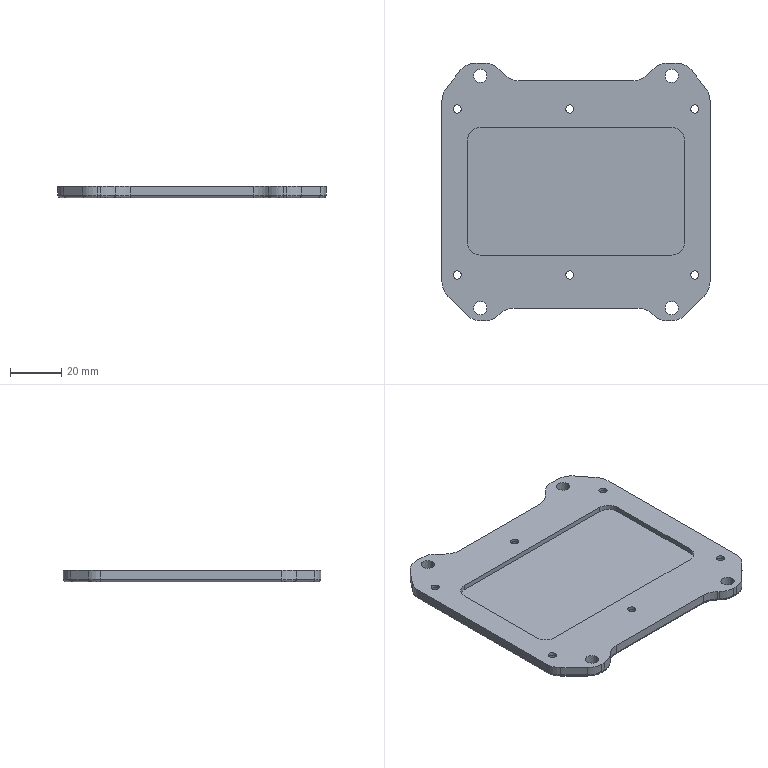NC program | NX | posted with a generic post | part box 105 x 101 x 4.5 mm
Whole program:
N10 G17 G21 G94 G90
(FLOOR_WALL_1 , TOOL : D80面刀)
N12 T01 M6
N14 G54
N16 G17 G0 G90 X-30.5 Y-95.5 S3500 M3
N18 G43 Z20. H1
N20 Z7.02
N22 G94 G1 Z4.02 F1000.
N24 Y-92.5
N26 Y92.5
N28 Y95.5
N30 Z7.02
N32 G0 Z20.
N34 X18.5 Y-95.5
N36 Z7.02
N38 G1 Z4.02
N40 Y-92.5
N42 Y92.5
N44 Y95.5
N46 Z7.02
N48 G0 Z20.
N50 X-30.5 Y-95.5
N52 Z6.04
N54 G1 Z3.04
N56 Y-92.5
N58 Y92.5
N60 Y95.5
N62 Z6.04
N64 G0 Z20.
N66 X18.5 Y-95.5
N68 Z6.04
N70 G1 Z3.04
N72 Y-92.5
N74 Y92.5
N76 Y95.5
N78 Z6.04
N80 G0 Z20.
N82 X-30.5 Y-95.5
N84 Z5.06
N86 G1 Z2.06
N88 Y-92.5
N90 Y92.5
N92 Y95.5
N94 Z5.06
N96 G0 Z20.
N98 X18.5 Y-95.5
N100 Z5.06
N102 G1 Z2.06
N104 Y-92.5
N106 Y92.5
N108 Y95.5
N110 Z5.06
N112 G0 Z20.
N114 X-30.5 Y-95.5
N116 Z4.08
N118 G1 Z1.08
N120 Y-92.5
N122 Y92.5
N124 Y95.5
N126 Z4.08
N128 G0 Z20.
N130 X18.5 Y-95.5
N132 Z4.08
N134 G1 Z1.08
N136 Y-92.5
N138 Y92.5
N140 Y95.5
N142 Z4.08
N144 G0 Z20.
N146 X-30.5 Y-95.5
N148 Z3.1
N150 G1 Z0.1
N152 Y-92.5
N154 Y92.5
N156 Y95.5
N158 Z3.1
N160 G0 Z20.
N162 X18.5 Y-95.5
N164 Z3.1
N166 G1 Z0.1
N168 Y-92.5
N170 Y92.5
N172 Y95.5
N174 Z3.1
N176 G0 Z20.
(FLOOR_WALL_1_COPY , TOOL : D80面刀)
N178 X-30.5 Y-95.5
N180 Z3.
N182 G1 Z0.
N184 Y-92.5
N186 Y92.5
N188 Y95.5
N190 Z3.
N192 G0 Z20.
N194 X18.5 Y-95.5
N196 Z3.
N198 G1 Z0.
N200 Y-92.5
N202 Y92.5
N204 Y95.5
N206 Z3.
N208 G0 Z20.
N210 M5
(PLANAR_MILL_2 , TOOL : D8-24-D8-60波刀)
N212 T02 M6
N214 G54
N216 G17 G0 G90 X2.576 Y17.778 S4500 M3
N218 G43 Z20. H2
N220 Z0.5
N222 G94 G1 Y20.35 Z0.365 F1500.
N224 X-3.124 Z0.066
N226 Y0. Z-1.
N228 Y-20.35
N230 X2.576
N232 Y20.35
N234 X-3.124
N236 Y0.
N238 X-9.124
N240 Y-26.35
N242 X8.576
N244 Y26.35
N246 X-9.124
N248 Y0.
N250 X-15.124
N252 Y-32.35
N254 X14.576
N256 Y32.35
N258 X-15.124
N260 Y0.
N262 X-21.124
N264 Y-37.5
N266 G3 X-20.274 Y-38.35 R0.85
N268 G1 X19.726
N270 G3 X20.576 Y-37.5 R0.85
N272 G1 Y37.5
N274 G3 X19.726 Y38.35 R0.85
N276 G1 X-20.274
N278 G3 X-21.124 Y37.5 R0.85
N280 G1 Y0.
N282 Z-0.5
N284 G0 Z20.
N286 X2.576 Y19.686
N288 Z-0.5
N290 G1 Y20.35 Z-0.535
N292 X-3.124 Z-0.834
N294 Y0. Z-1.9
N296 Y-20.35
N298 X2.576
N300 Y20.35
N302 X-3.124
N304 Y0.
N306 X-9.124
N308 Y-26.35
N310 X8.576
N312 Y26.35
N314 X-9.124
N316 Y0.
N318 X-15.124
N320 Y-32.35
N322 X14.576
N324 Y32.35
N326 X-15.124
N328 Y0.
N330 X-21.124
N332 Y-37.5
N334 G3 X-20.274 Y-38.35 R0.85
N336 G1 X19.726
N338 G3 X20.576 Y-37.5 R0.85
N340 G1 Y37.5
N342 G3 X19.726 Y38.35 R0.85
N344 G1 X-20.274
N346 G3 X-21.124 Y37.5 R0.85
N348 G1 Y0.
N350 Z-1.4
N352 G0 Z20.
N354 M5
(PLANAR_MILL_2_COPY , TOOL : D8-25-D8-60-3T-FINISH)
N356 T03 M6
N358 G54
N360 G17 G0 G90 X-3.374 Y0.303 S3500 M3
N362 G43 Z20. H3
N364 Z0.5
N366 G94 G1 Y-20.6 Z-0.595 F800.
N368 X2.826 Z-0.92
N370 Y0. Z-2.
N372 Y20.6
N374 X-3.374
N376 Y-20.6
N378 X2.826
N380 Y0.
N382 X8.826
N384 Y26.6
N386 X-9.374
N388 Y-26.6
N390 X8.826
N392 Y0.
N394 X14.826
N396 Y32.6
N398 X-15.374
N400 Y-32.6
N402 X14.826
N404 Y0.
N406 X20.826
N408 Y37.5
N410 G3 X19.726 Y38.6 R1.1
N412 G1 X-20.274
N414 G3 X-21.374 Y37.5 R1.1
N416 G1 Y-37.5
N418 G3 X-20.274 Y-38.6 R1.1
N420 G1 X19.726
N422 G3 X20.826 Y-37.5 R1.1
N424 G1 Y0.
N426 Z-1.5
N428 G0 Z20.
N430 M5
(PLANAR_MILL_3 , TOOL : 倒角D8-90度)
N432 T05 M6
N434 G54
N436 G17 G0 G90 X19.726 Y-2. S3500 M3
N438 G43 Z20. H5
N440 Z1.
N442 G94 G1 Z-1. F1000.
N444 X21.726
N446 G3 X23.726 Y0. R2.
N448 G1 Y37.5
N450 G3 X19.726 Y41.5 R4.
N452 G1 X-20.274
N454 G3 X-24.274 Y37.5 R4.
N456 G1 Y-37.5
N458 G3 X-20.274 Y-41.5 R4.
N460 G1 X19.726
N462 G3 X23.726 Y-37.5 R4.
N464 G1 Y0.
N466 G3 X21.726 Y2. R2.
N468 G1 X19.726
N470 Z1.
N472 G0 Z20.
(PLANAR_MILL_3_COPY , TOOL : 倒角D8-90度)
N474 X1.726 Y-57.5
N476 Z2.
N478 G1 Z-1.
N480 Y-55.5
N482 G3 X-0.274 Y-53.5 R2.
N484 G1 X-35.734
N486 G2 X-41.293 Y-51.578 R9.
N488 G1 X-48.059 Y-46.264
N490 G2 X-51.5 Y-39.186 R9.
N492 G1 Y-35.814
N494 G2 X-48.864 Y-29.45 R9.
N496 G1 X-46.55 Y-27.136
N498 G3 X-44.5 Y-22.186 R7.
N500 G1 Y22.186
N502 G3 X-46.55 Y27.136 R7.
N504 G1 X-48.864 Y29.45
N506 G2 X-51.5 Y35.814 R9.
N508 G1 Y39.186
N510 G2 X-48.059 Y46.264 R9.
N512 G1 X-41.293 Y51.578
N514 G2 X-35.734 Y53.5 R9.
N516 G1 X35.186
N518 G2 X41.55 Y50.864 R9.
N520 G1 X48.864 Y43.55
N522 G2 X51.5 Y37.186 R9.
N524 G1 Y35.814
N526 G2 X48.864 Y29.45 R9.
N528 G1 X48.55 Y29.136
N530 G3 X46.5 Y24.186 R7.
N532 G1 Y-24.186
N534 G3 X48.55 Y-29.136 R7.
N536 G1 X48.864 Y-29.45
N538 G2 X51.5 Y-35.814 R9.
N540 G1 Y-37.186
N542 G2 X48.864 Y-43.55 R9.
N544 G1 X41.55 Y-50.864
N546 G2 X35.186 Y-53.5 R9.
N548 G1 X-0.274
N550 G3 X-2.274 Y-55.5 R2.
N552 G1 Y-57.5
N554 Z2.
N556 G0 Z20.
(SPOT_DRILLING_2 , TOOL : 倒角D8-90度)
N558 X-45.5 Y-37.5 S2500
N560 G81 G98 Z-2.7 F200. R3.
N562 Y37.5
N564 X45.5
N566 Y-37.5
N568 X-32.5 Y-46.5 Z-1.7
N570 Y-2.5
N572 Y46.5
N574 X32.5
N576 Y-2.5
N578 Y-46.5
N580 G80
N582 M5
N584 M2